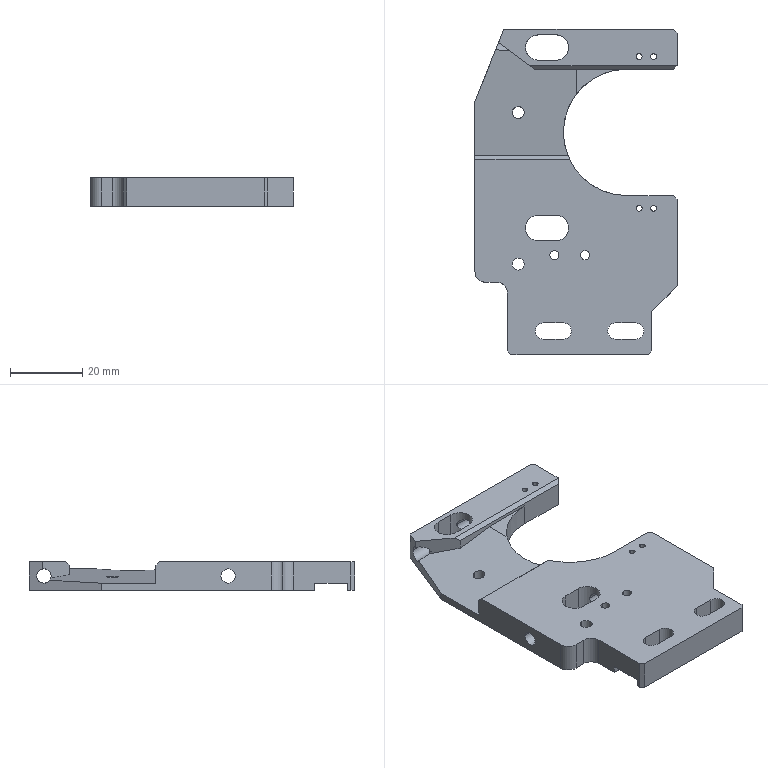NC program | NX | posted with a generic post | part box 56 x 90 x 8 mm
Whole program:
N10 G17 G21 G94 G90
(FLOOR_WALL_COPY , TOOL : D63)
N12 T03 M6
N14 G54
N16 G17 G0 G90 X79.5 Y-27.997 S6500 M3
N18 G43 Z30. H3
N20 Z4.
N22 G94 G1 Z1. F1500.
N24 X76.5
N26 X-76.5
N28 Y-22.258
N30 Y2.8
N32 X76.5
N34 X79.5
N36 Z4.
N38 G0 Z30.
N40 Y-27.997
N42 Z3.
N44 G1 Z0.
N46 X76.5
N48 X-76.5
N50 Y-22.258
N52 Y2.8
N54 X76.5
N56 X79.5
N58 Z3.
N60 G0 Z30.
N62 M5
N64 M2